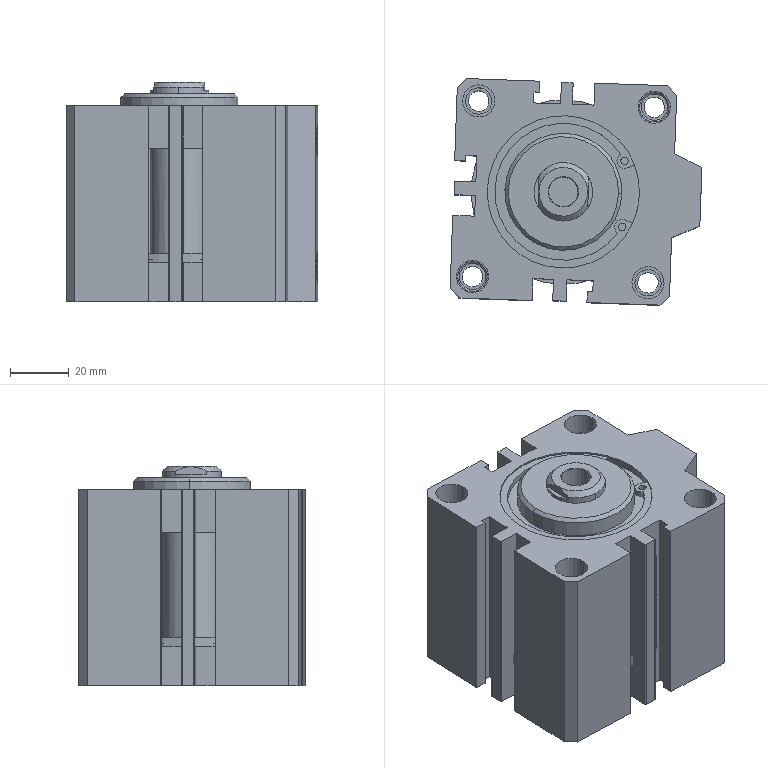Part | SolidWorks | 2 solids | 211 faces | box 86.017 x 77.396 x 75.017 mm | volume 256074 mm3 | cylinder 101 | plane 88 | cone 14 | spline 8 | commonest cylinder face diameters 11 x44 9 x16 0.6 x8 7 x8 63 x5 2.6 x4